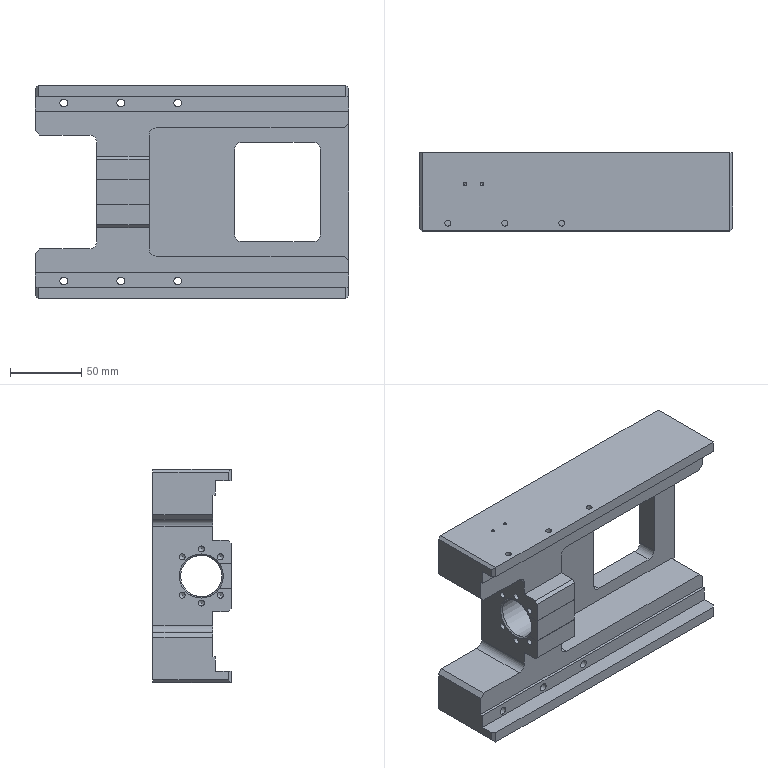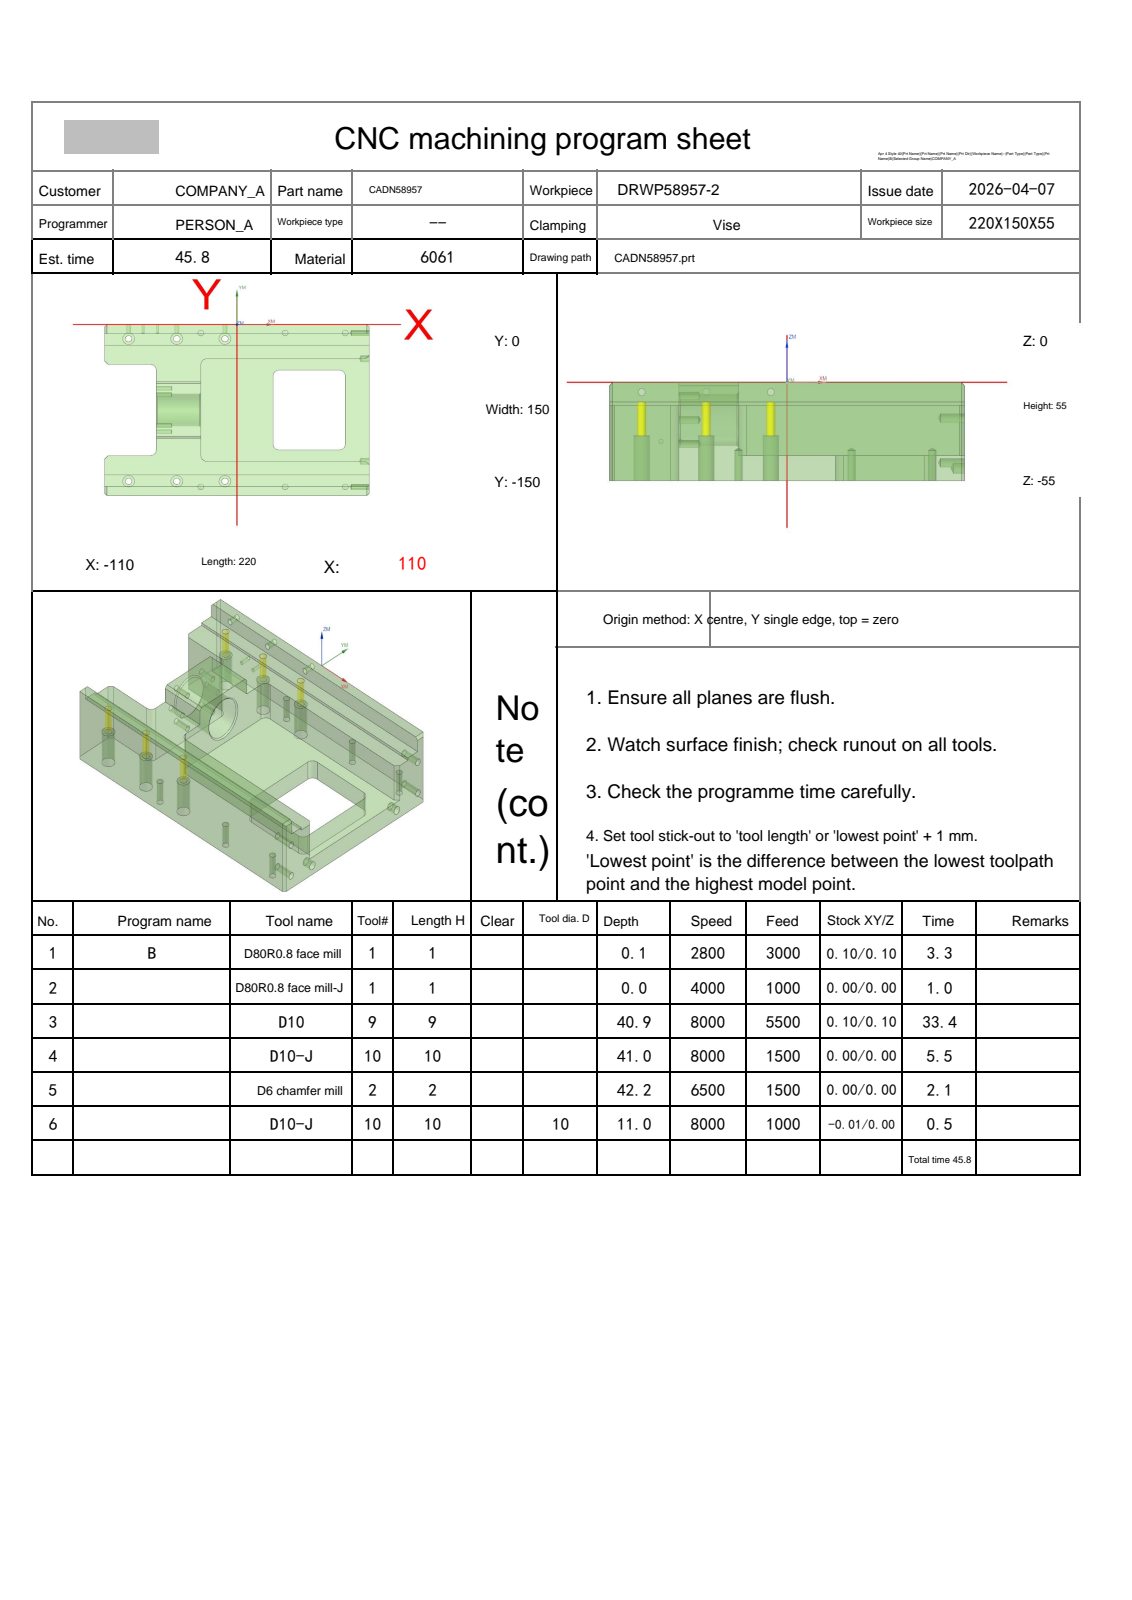NC program | NX | posted by the shop | part box 220 x 55 x 150 mm
Lines 209 to 1303 of 15484:
N3 T09 M06
(D10  D=10. R=0. H=09 ce=0.10 di=0.10)
G00 G90 G54 X124.5 Y-57.103 M03 S8000
G43 H09 Z14.5
M08
Z.519
G01 Z-.681 F5500.
X117.071 Y-57.1
X117.069
G03 X110.069 Y-64.097 I0.0 J-7.
G01 X110.05 Y-115.854
X110.06 Y-115.933
X109.985 Y-115.973
X109.925 Y-115.92
X109.712 Y-115.776
X108.83 Y-115.325
X108.229 Y-115.133
X107.955 Y-115.071
X107.072 Y-114.98
X-20.611 Y-114.978
G02 X-21.301 Y-114.701 I0.0 J1.
G01 X-24.423 Y-111.722
G03 X-25.113 Y-111.446 I-.69 J-.723
G01 X-25.209 Y-111.45
X-33.928 Y-112.288
G02 X-34.167 Y-112.299 I-.239 J2.489
X-36.667 Y-109.799 I0.0 J2.5
X-34.406 Y-107.311 I2.5 J0.0
G01 X-23.365 Y-106.25
G02 X-23.126 Y-106.239 I.239 J-2.489
X-20.626 Y-108.739 I0.0 J-2.5
X-21.254 Y-110.396 I-2.5 J0.0
G01 X-24.533 Y-114.678
G02 X-25.309 Y-115.07 I-.794 J.608
G01 X-25.877 Y-115.08
X-29.442
X-30.06 Y-115.142
X-29.576 Y-116.808
X-29.375 Y-117.251
X-29.126 Y-117.68
X-28.494 Y-118.464
X-28.401 Y-118.556
X-27.617 Y-119.166
X-27.132 Y-119.434
X-26.742 Y-119.601
X-25.862 Y-119.843
X-24.981 Y-119.92
X107.
X107.057 Y-119.943
X110.057 Y-122.943
X110.08 Y-123.
Y-126.698
X110.079 Y-127.517
X110.08 Y-135.647
Y-136.418
Y-136.823
G02 X114.225 Y-139.047 I-.107 J-5.175
X115.158 Y-142.351 I-5.386 J-3.304
X115.151 Y-142.651 I-6.318 J0.0
G01 Y-148.
X115.127 Y-148.057
X113.936 Y-149.248
X113.823
Y-142.
G03 X108.893 Y-136.904 I-5.121 J-.021
G01 X108.343 Y-136.832
X108.169 Y-136.822
X107.968 Y-136.821
X-104.399
X-105.291
X-107.968
X-108.173 Y-136.822
X-108.349 Y-136.832
X-108.894 Y-136.904
G03 X-113.823 Y-142. I.192 J-5.117
G01 Y-149.248
X-113.931 Y-149.249
X-115.127 Y-148.046
X-115.151 Y-147.99
Y-142.647
X-115.13 Y-141.755
G02 X-110.08 Y-136.824 I5.205 J-.279
G01 Y-136.418
Y-135.647
X-110.079 Y-127.517
X-110.08 Y-126.698
Y-118.
X-110.057 Y-117.943
X-107.057 Y-114.943
X-107. Y-114.92
X-72.278
X-70.917 Y-114.862
X-69.636 Y-114.315
X-69.279 Y-114.099
X-68.759 Y-113.701
X-68.513 Y-113.471
X-68.283 Y-113.224
X-67.881 Y-112.691
X-67.677 Y-112.349
X-67.136 Y-111.071
X-67.08 Y-109.713
Y-105.264
X-67.082 Y-105.086
X-67.081 Y-103.823
X-67.001
X-66.998
X-66.997
X-66.921 Y-103.824
X-37.336 Y-103.823
G02 X-36.336 Y-104.823 I0.0 J-1.
G01 X-36.35 Y-104.989
X-37.197 Y-110.005
X-37.211 Y-110.171
G03 X-36.775 Y-110.997 I1. J0.0
G02 X-36.339 Y-111.823 I-.564 J-.826
X-36.428 Y-112.235 I-1. J0.0
G03 X-37.06 Y-115.142 I6.368 J-2.907
X-36.782 Y-117.097 I7. J0.0
G01 X-36.157 Y-119.243
X-35.605 Y-120.461
X-34.911 Y-121.657
X-33.689 Y-123.173
X-33.019 Y-123.831
X-31.484 Y-125.027
X-30.211 Y-125.73
X-29.062 Y-126.223
X-27.105 Y-126.762
X-25.284 Y-126.92
X102.083
G02 X103.079 Y-127.916 I-.003 J-1.
G01 Y-128.825
G02 X102.083 Y-129.821 I-1. J.003
G01 X-64.065
G02 X-64.758 Y-129.542 I0.0 J1.
G01 X-66.167 Y-128.188
G03 X-66.65 Y-127.931 I-.693 J-.721
G02 X-68.627 Y-125.486 I.523 J2.445
X-66.82 Y-123.084 I2.5 J0.0
G01 X-59.894 Y-121.087
G02 X-59.202 Y-120.989 I.693 J-2.402
X-56.702 Y-123.489 I0.0 J-2.5
X-58.509 Y-125.891 I-2.5 J0.0
G01 X-64.219 Y-127.538
G03 X-64.7 Y-127.846 I.277 J-.961
G01 X-66.101 Y-129.474
G02 X-66.859 Y-129.821 I-.758 J.653
G01 X-102.083
G02 X-103.079 Y-128.825 I.003 J1.
G01 Y-127.514
X-103.08 Y-126.695
Y-122.916
G02 X-102.084 Y-121.92 I1. J-.004
G01 X-72.128
X-70.619 Y-121.856
G03 X-68.168 Y-121.299 I-.299 J6.994
G01 X-66.436 Y-120.559
X-65.332 Y-119.893
X-64.228 Y-119.049
X-63.548 Y-118.412
X-62.912 Y-117.726
X-62.065 Y-116.605
X-61.419 Y-115.522
X-60.69 Y-113.799
G03 X-60.167 Y-111.725 I-6.446 J2.729
G02 X-59.175 Y-110.823 I.995 J-.097
G01 X-40.813
G02 X-40.114 Y-111.523 I0.0 J-.7
X-40.151 Y-111.748 I-.7 J0.0
G01 X-43.004 Y-120.119
G03 X-43.057 Y-120.442 I.947 J-.322
X-43.018 Y-120.721 I1. J0.0
G01 X-42.778 Y-121.546
G02 X-42.739 Y-121.821 I-.961 J-.275
X-43.735 Y-122.821 I-1. J0.0
G01 X-55.984
G02 X-56.98 Y-121.821 I.004 J1.
X-56.78 Y-121.222 I1. J0.0
G01 X-56.249 Y-120.518
X-55.161 Y-118.695
X-55.048 Y-118.429
G02 X-54.133 Y-117.823 I.919 J-.394
G01 X-46.706
G03 X-46.094 Y-117.613 I0.0 J1.
G01 X-37.808 Y-111.189
G03 X-37.421 Y-110.399 I-.613 J.79
G01 X-37.435 Y-110.233
X-38.322 Y-104.989
X-38.336 Y-104.823
G02 X-37.336 Y-103.823 I1. J0.0
G01 X-30.
G03 X-24.905 Y-98.909 I-.049 J5.149
G01 X-24.865 Y-98.686
X-24.822 Y-98.143
X-24.821 Y-97.253
Y-52.747
X-24.822 Y-51.851
X-24.866 Y-51.305
X-24.905 Y-51.091
G03 X-30. Y-46.177 I-5.144 J-.235
G01 X-66.921
X-66.997
X-66.998
X-67.001
X-67.002
X-67.081
X-67.082 Y-44.898
X-67.08 Y-40.287
X-67.136 Y-38.929
X-67.677 Y-37.651
X-67.881 Y-37.309
X-68.283 Y-36.777
X-68.76 Y-36.298
X-69.279 Y-35.901
X-69.636 Y-35.685
X-70.917 Y-35.138
X-72.278 Y-35.08
X-107.
X-107.057 Y-35.057
X-110.057 Y-32.057
X-110.08 Y-32.
Y-23.302
X-110.079 Y-22.483
X-110.08 Y-14.353
Y-13.176
G02 X-112.672 Y-12.396 I.155 J5.21
X-115.13 Y-8.242 I2.748 J4.43
G01 X-115.151 Y-6.461
Y-2.
X-115.127 Y-1.943
X-113.935 Y-.751
X-113.823 Y-.752
X-113.822 Y-8.068
G03 X-108.895 Y-13.096 I5.12 J.088
G01 X-108.343 Y-13.168
X-108.169 Y-13.178
X-7.311 Y-13.179
X99.045
X99.937 Y-13.18
X101.722
X102.168
X102.614
X103.507
X104.399
X105.291
X108.004 Y-13.177
X108.173 Y-13.178
X108.349 Y-13.168
X108.894 Y-13.096
G03 X113.823 Y-8. I-.192 J5.117
G01 Y-.752
X113.932
X115.127 Y-1.954
X115.151 Y-2.01
Y-6.462
X115.13 Y-8.245
G02 X113. Y-12.174 I-5.206 J.28
X110.08 Y-13.177 I-3.077 J4.209
G01 X110.079 Y-22.483
X110.08 Y-23.302
Y-26.967
X113. Y-29.888
Y-31.328
X110.698 Y-33.63
X110.143 Y-34.118
X110.08 Y-34.166
X110.07 Y-61.083
G02 X109.651 Y-61.896 I-1. J.001
G01 X103.486 Y-66.296
G03 X103.068 Y-67.109 I.581 J-.814
G01 X103.053 Y-106.984
G02 X102.057 Y-107.98 I-1. J.004
G01 X-19.858 Y-107.978
G02 X-20.854 Y-106.978 I.003 J1.
X-20.632 Y-106.349 I1. J0.0
G03 X-17.951 Y-99.781 I-9.418 J7.676
X-17.887 Y-99.24 I-6.994 J1.101
G01 X-17.844 Y-98.703
G03 X-17.822 Y-98.143 I-7.058 J.56
G01 Y-51.857
G03 X-17.844 Y-51.297 I-7.08 J0.0
G01 X-17.887 Y-50.76
G03 X-17.951 Y-50.219 I-7.058 J-.56
X-29.966 Y-39.177 I-12.099 J-1.108
G01 X-59.175
G02 X-60.167 Y-38.275 I.003 J1.
G03 X-60.69 Y-36.201 I-6.969 J-.655
G01 X-61.419 Y-34.478
X-62.065 Y-33.395
X-62.368 Y-32.995
X-62.985 Y-32.177
X-64.133 Y-31.024
X-65.332 Y-30.107
X-66.436 Y-29.441
X-68.168 Y-28.701
G03 X-70.619 Y-28.144 I-2.749 J-6.437
G01 X-72.128 Y-28.08
X-102.084
G02 X-103.08 Y-27.083 I.004 J1.
G01 Y-23.305
X-103.079 Y-22.486
Y-21.174
G02 X-102.083 Y-20.178 I1. J-.003
G01 X-66.86
G02 X-66.102 Y-20.526 I0.0 J-1.
G01 X-64.7 Y-22.153
G03 X-64.22 Y-22.462 I.758 J.653
G01 X-58.509 Y-24.108
G02 X-56.702 Y-26.511 I-.693 J-2.402
X-59.202 Y-29.011 I-2.5 J0.0
X-59.894 Y-28.913 I0.0 J2.5
G01 X-66.82 Y-26.915
G02 X-68.627 Y-24.513 I.693 J2.402
X-66.651 Y-22.069 I2.5 J0.0
G03 X-66.167 Y-21.812 I-.209 J.978
G01 X-64.758 Y-20.457
G02 X-64.065 Y-20.178 I.693 J-.721
G01 X-7.311 Y-20.179
X99.041
X99.933 Y-20.18
X101.721
X102.083
G02 X103.079 Y-21.177 I-.004 J-1.
G01 Y-22.486
X103.08 Y-23.305
Y-26.967
G03 X103.83 Y-30.12 I7. J0.0
G02 X103.935 Y-30.567 I-.895 J-.447
X103.83 Y-31.014 I-1. J0.0
G03 X103.08 Y-34.163 I6.25 J-3.152
G01 X103.07 Y-61.081
G02 X102.651 Y-61.894 I-1. J.001
G01 X96.486 Y-66.294
G03 X96.068 Y-67.106 I.581 J-.814
G01 X96.056 Y-99.984
G02 X95.06 Y-100.98 I-1. J.004
G01 X-9.924 Y-100.978
G02 X-10.92 Y-99.978 I.004 J1.
G01 X-10.917 Y-99.896
X-10.866 Y-99.257
G03 X-10.822 Y-98.143 I-14.036 J1.114
G01 Y-51.857
G03 X-10.866 Y-50.743 I-14.08 J0.0
G01 X-10.909 Y-50.206
G03 X-11. Y-49.368 I-14.036 J-1.114
X-29.942 Y-32.177 I-19.049 J-1.959
G01 X-54.133
G02 X-55.048 Y-31.571 I.004 J1.
G01 X-55.161 Y-31.305
X-56.249 Y-29.482
X-56.78 Y-28.778
G02 X-56.98 Y-28.178 I.801 J.599
X-55.984 Y-27.178 I1. J0.0
G01 X-18.168 Y-27.179
G02 X-17.401 Y-27.538 I0.0 J-1.
G01 X-16.08 Y-29.12
G03 X-15.642 Y-29.424 I.768 J.641
G01 X-10.619 Y-31.176
G02 X-8.942 Y-33.536 I-.823 J-2.361
X-11.442 Y-36.036 I-2.5 J0.0
X-12.266 Y-35.897 I0.0 J2.5
G01 X-18.423 Y-33.749
G02 X-20.099 Y-31.389 I.823 J2.361
X-17.97 Y-28.916 I2.5 J0.0
G03 X-17.437 Y-28.658 I-.148 J.989
G01 X-16.139 Y-27.448
G02 X-15.457 Y-27.179 I.682 J-.731
G01 X-7.311
X95.133
G02 X96.125 Y-28.094 I-.004 J-1.
G03 X96.49 Y-30.331 I13.955 J1.127
G02 X96.518 Y-30.567 I-.972 J-.236
X96.49 Y-30.803 I-1. J0.0
G03 X96.08 Y-34.166 I13.59 J-3.363
G01 Y-34.179
X96.07 Y-61.078
G02 X95.651 Y-61.891 I-1. J.001
G01 X89.486 Y-66.291
G03 X89.068 Y-67.104 I.581 J-.814
G01 X89.058 Y-92.984
G02 X88.063 Y-93.98 I-1. J.005
G01 X-2.826 Y-93.978
G02 X-3.822 Y-92.983 I.004 J1.
G01 Y-51.857
G03 X-3.888 Y-50.19 I-21.08 J0.0
G01 X-3.931 Y-49.652
G03 X-4.05 Y-48.527 I-21.014 J-1.668
X-9.03 Y-35.77 I-25.999 J-2.799
G02 X-9.224 Y-35.179 I.807 J.591
X-8.228 Y-34.179 I1. J0.0
G01 X-7.311
X88.084
G02 X89.08 Y-35.175 I-.004 J-1.
G01 X89.07 Y-61.076
G02 X88.651 Y-61.888 I-1. J.001
G01 X82.487 Y-66.288
G03 X82.068 Y-67.101 I.581 J-.814
G01 X82.061 Y-85.985
G02 X81.066 Y-86.979 I-1. J.005
G01 X4.173 Y-86.978
G02 X3.178 Y-85.983 I.005 J1.
G01 Y-51.856
G03 X3.09 Y-49.636 I-28.08 J0.0
G01 X3.048 Y-49.098
G03 X2.9 Y-47.69 I-27.992 J-2.222
X1.887 Y-42.442 I-32.949 J-3.637
G02 X1.852 Y-42.179 I.965 J.263
X2.847 Y-41.179 I1. J0.0
G01 X81.082
G02 X82.077 Y-42.174 I-.005 J-1.
G01 X82.07 Y-61.073
G02 X81.651 Y-61.886 I-1. J.001
G01 X75.487 Y-66.286
G03 X75.068 Y-67.099 I.581 J-.814
G01 X75.063 Y-78.985
G02 X74.068 Y-79.979 I-1. J.005
G01 X11.173 Y-79.978
G02 X10.178 Y-78.983 I.005 J1.
G01 Y-51.856
G03 X10.081 Y-49.248 I-35.08 J-.001
G01 X10.079 Y-49.179
G02 X11.074 Y-48.179 I1. J0.0
G01 X74.079
G02 X75.074 Y-49.174 I-.005 J-1.
G01 X75.07 Y-61.07
G02 X74.651 Y-61.883 I-1. J.001
G01 X68.487 Y-66.283
G03 X68.068 Y-67.096 I.581 J-.814
G01 X68.066 Y-71.985
G02 X67.071 Y-72.979 I-1. J.005
G01 X18.173
G02 X17.178 Y-71.984 I.005 J1.
G01 Y-56.174
G02 X18.173 Y-55.179 I1. J-.005
G01 X67.077
G02 X68.072 Y-56.174 I-.005 J-1.
G01 X68.07 Y-60.957
G02 X67.507 Y-61.855 I-1. J.001
G01 X61.508 Y-64.771
G03 X61.007 Y-65.325 I.438 J-.899
G02 X60.074 Y-65.979 I-.938 J.345
G01 X25.173
G02 X24.178 Y-64.984 I.005 J1.
G01 Y-63.174
G02 X25.173 Y-62.179 I1. J-.005
G01 X60.074
G02 X61.069 Y-63.174 I-.005 J-1.
G01 Y-64.079
Y-64.579
Y-64.582
G03 X68.066 Y-71.582 I7. J0.0
G01 Z.519
G00 Z3.
G01 X124.5 Y-57.103 F6000.
G00 Z-.163
G01 Z-1.363 F5500.
X117.071 Y-57.1
X117.069
G03 X110.069 Y-64.097 I0.0 J-7.
G01 X110.05 Y-115.854
X110.06 Y-115.933
X109.985 Y-115.973
X109.925 Y-115.92
X109.712 Y-115.776
X108.83 Y-115.325
X108.229 Y-115.133
X107.955 Y-115.071
X107.072 Y-114.98
X-20.031 Y-114.978
G02 X-20.718 Y-114.705 I0.0 J1.
G01 X-23.701 Y-111.886
G03 X-24.387 Y-111.612 I-.687 J-.727
G01 X-24.504 Y-111.619
X-34.254 Y-112.76
G02 X-34.545 Y-112.777 I-.291 J2.483
X-37.045 Y-110.277 I0.0 J2.5
X-34.835 Y-107.794 I2.5 J0.0
G01 X-22.821 Y-106.388
G02 X-22.531 Y-106.371 I.291 J-2.483
X-20.031 Y-108.871 I0.0 J-2.5
X-20.667 Y-110.538 I-2.5 J0.0
G01 X-23.752 Y-114.584
G02 X-24.547 Y-114.978 I-.795 J.606
G01 X-24.819
X-24.943 Y-115.053
X-24.983 Y-115.064
X-25.877 Y-115.08
X-29.442
X-30.06 Y-115.142
X-29.576 Y-116.808
X-29.375 Y-117.251
X-29.126 Y-117.68
X-28.494 Y-118.464
X-28.401 Y-118.556
X-27.617 Y-119.166
X-27.132 Y-119.434
X-26.742 Y-119.601
X-25.862 Y-119.843
X-24.981 Y-119.92
X107.
X107.057 Y-119.943
X110.057 Y-122.943
X110.08 Y-123.
Y-126.698
X110.079 Y-127.517
X110.08 Y-136.418
Y-136.823
G02 X114.225 Y-139.047 I-.107 J-5.175
X115.158 Y-142.351 I-5.386 J-3.304
X115.151 Y-142.651 I-6.318 J0.0
G01 Y-148.
X115.127 Y-148.057
X114.617 Y-148.567
X114.504
Y-142.
G03 X109.383 Y-136.9 I-5.121 J-.021
G01 X109.362
X108.878
X108.343 Y-136.832
X108.169 Y-136.822
X107.968 Y-136.821
X-104.399
X-105.292
X-107.968
X-108.173 Y-136.822
X-108.349 Y-136.832
X-108.878 Y-136.9
X-109.367
G03 X-114.504 Y-142.037 I0.0 J-5.137
G01 Y-148.567
X-114.609
X-115.127 Y-148.046
X-115.151 Y-147.99
Y-142.647
X-115.13 Y-141.755
G02 X-110.08 Y-136.824 I5.205 J-.279
G01 Y-136.418
X-110.079 Y-127.517
X-110.08 Y-126.698
Y-118.
X-110.057 Y-117.943
X-107.057 Y-114.943
X-107. Y-114.92
X-72.278
X-70.917 Y-114.862
X-69.636 Y-114.315
X-69.279 Y-114.099
X-68.759 Y-113.701
X-68.513 Y-113.471
X-68.283 Y-113.224
X-67.881 Y-112.691
X-67.677 Y-112.349
X-67.136 Y-111.071
X-67.08 Y-109.713
Y-105.264
X-67.082 Y-105.086
X-67.081 Y-104.504
X-67.051
X-67.05 Y-104.505
X-67.001 Y-104.504
X-66.921 Y-104.505
X-37.609 Y-104.504
G02 X-36.609 Y-105.504 I0.0 J-1.
G01 X-36.623 Y-105.671
X-37.471 Y-110.686
X-37.485 Y-110.852
G03 X-37.049 Y-111.678 I1. J0.0
G02 X-36.613 Y-112.504 I-.564 J-.826
X-36.668 Y-112.831 I-1. J0.0
G03 X-37.06 Y-115.142 I6.607 J-2.311
X-36.782 Y-117.097 I7. J0.0
G01 X-36.157 Y-119.243
X-35.605 Y-120.461
X-34.911 Y-121.657
X-33.689 Y-123.173
X-33.019 Y-123.831
X-31.484 Y-125.027
X-30.211 Y-125.73
X-29.062 Y-126.223
X-27.105 Y-126.762
X-25.284 Y-126.92
X102.083
G02 X103.079 Y-127.916 I-.003 J-1.
G01 Y-128.825
G02 X102.083 Y-129.821 I-1. J.003
G01 X-64.065
G02 X-64.758 Y-129.542 I0.0 J1.
G01 X-66.167 Y-128.188
G03 X-66.65 Y-127.931 I-.693 J-.721
G02 X-68.627 Y-125.486 I.523 J2.445
X-66.82 Y-123.084 I2.5 J0.0
G01 X-59.894 Y-121.087
G02 X-59.202 Y-120.989 I.693 J-2.402
X-56.702 Y-123.489 I0.0 J-2.5
X-58.509 Y-125.891 I-2.5 J0.0
G01 X-64.219 Y-127.538
G03 X-64.7 Y-127.846 I.277 J-.961
G01 X-66.101 Y-129.474
G02 X-66.859 Y-129.821 I-.758 J.653
G01 X-102.083
G02 X-103.079 Y-128.825 I.003 J1.
G01 Y-127.514
X-103.08 Y-126.695
Y-122.916
G02 X-102.084 Y-121.92 I1. J-.004
G01 X-72.128
X-70.619 Y-121.856
G03 X-68.168 Y-121.299 I-.299 J6.994
G01 X-66.436 Y-120.559
X-65.332 Y-119.893
X-64.228 Y-119.049
X-63.548 Y-118.412
X-62.912 Y-117.726
X-62.065 Y-116.605
X-61.419 Y-115.522
X-60.69 Y-113.799
G03 X-60.249 Y-112.322 I-6.446 J2.729
G02 X-59.269 Y-111.504 I.983 J-.182
G01 X-41.044
G02 X-40.344 Y-112.204 I0.0 J-.7
G01 X-40.373 Y-112.401
X-42.835 Y-120.785
G03 X-42.876 Y-121.067 I.96 J-.281
X-42.836 Y-121.346 I1. J0.0
G01 X-42.778 Y-121.546
G02 X-42.739 Y-121.821 I-.961 J-.275
X-43.735 Y-122.821 I-1. J0.0
G01 X-55.984
G02 X-56.98 Y-121.821 I.004 J1.
X-56.78 Y-121.222 I1. J0.0
G01 X-56.249 Y-120.518
X-55.336 Y-118.988
G02 X-54.483 Y-118.504 I.857 J-.516
G01 X-46.564
G03 X-45.933 Y-118.28 I0.0 J1.
G01 X-38.061 Y-111.871
G03 X-37.692 Y-111.096 I-.632 J.775
G01 X-37.706 Y-110.93
X-38.595 Y-105.671
X-38.609 Y-105.504
G02 X-37.609 Y-104.504 I1. J0.0
G01 X-30.
G03 X-24.9 Y-99.383 I-.021 J5.121
G01 Y-99.362
Y-98.88
X-24.865 Y-98.686
X-24.822 Y-98.143
X-24.821 Y-97.253
Y-52.747
X-24.822 Y-51.851
X-24.866 Y-51.305
X-24.9 Y-51.12
Y-50.615
G03 X-30. Y-45.496 I-5.121 J-.002
G01 X-66.921
X-67.001
Y-45.495
X-67.081 Y-45.496
X-67.082 Y-44.898
X-67.08 Y-40.287
X-67.136 Y-38.929
X-67.677 Y-37.651
X-67.881 Y-37.309
X-68.283 Y-36.777
X-68.76 Y-36.298
X-69.279 Y-35.901
X-69.636 Y-35.685
X-70.917 Y-35.138
X-72.278 Y-35.08
X-107.
X-107.057 Y-35.057
X-110.057 Y-32.057
X-110.08 Y-32.
Y-23.302
X-110.079 Y-22.483
X-110.08 Y-14.461
Y-13.176
G02 X-115.13 Y-8.242 I.155 J5.21
G01 X-115.151 Y-6.461
Y-2.
X-115.127 Y-1.943
X-114.617 Y-1.433
X-114.504
Y-7.963
G03 X-109.367 Y-13.1 I5.137 J0.0
G01 X-108.879
X-108.343 Y-13.168
X-108.169 Y-13.178
X-7.311 Y-13.179
X99.045
X99.937 Y-13.18
X101.722
X102.614
X103.507
X104.399
X105.291
X108.004 Y-13.177
X108.173 Y-13.178
X108.349 Y-13.168
X108.879 Y-13.1
X109.362
X109.383
G03 X114.504 Y-8. I0.0 J5.121
G01 Y-1.433
X114.609
X115.127 Y-1.954
X115.151 Y-2.01
Y-6.462
X115.13 Y-8.245
G02 X110.08 Y-13.176 I-5.206 J.28
G01 X110.079 Y-22.483
X110.08 Y-23.302
Y-26.967
X113. Y-29.888
Y-31.328
X110.698 Y-33.63
X110.143 Y-34.118
X110.08 Y-34.166
X110.07 Y-61.083
G02 X109.651 Y-61.896 I-1. J.001
G01 X103.486 Y-66.296
G03 X103.068 Y-67.109 I.581 J-.814
G01 X103.053 Y-106.984
G02 X102.057 Y-107.98 I-1. J.004
G01 X-19.325 Y-107.978
G02 X-20.322 Y-106.978 I.004 J1.
X-20.139 Y-106.402 I1. J0.0
G03 X-17.9 Y-99.388 I-9.882 J7.019
G01 X-17.881 Y-99.17
X-17.844 Y-98.703
G03 X-17.822 Y-98.143 I-7.058 J.56
G01 Y-51.857
G03 X-17.844 Y-51.297 I-7.08 J0.0
G01 X-17.887 Y-50.76
X-17.9 Y-50.612
G03 X-29.986 Y-38.496 I-12.121 J-.005
G01 X-59.269
G02 X-60.249 Y-37.678 I.003 J1.
G03 X-60.69 Y-36.201 I-6.887 J-1.251
G01 X-61.419 Y-34.478
X-62.065 Y-33.395
X-62.984 Y-32.178
X-64.133 Y-31.024
X-65.332 Y-30.107
X-66.436 Y-29.441
X-68.168 Y-28.701
G03 X-70.619 Y-28.144 I-2.749 J-6.437
G01 X-72.128 Y-28.08
X-102.084
G02 X-103.08 Y-27.084 I.003 J1.
G01 Y-23.305
X-103.079 Y-22.486
Y-21.174
G02 X-102.083 Y-20.178 I1. J-.003
G01 X-66.86
G02 X-66.102 Y-20.526 I0.0 J-1.
G01 X-64.7 Y-22.153
G03 X-64.22 Y-22.462 I.758 J.653
G01 X-58.509 Y-24.108
G02 X-56.702 Y-26.511 I-.693 J-2.402
X-59.202 Y-29.011 I-2.5 J0.0
X-59.894 Y-28.913 I0.0 J2.5
G01 X-66.82 Y-26.915
G02 X-68.627 Y-24.513 I.693 J2.402
X-66.651 Y-22.069 I2.5 J0.0
G03 X-66.167 Y-21.812 I-.209 J.978
G01 X-64.758 Y-20.457
G02 X-64.065 Y-20.178 I.693 J-.721
G01 X-7.311 Y-20.179
X99.041
X99.933 Y-20.18
X101.721
X102.083
G02 X103.079 Y-21.177 I-.004 J-1.
G01 Y-22.486
X103.08 Y-23.305
Y-26.967
G03 X103.83 Y-30.12 I7. J0.0
G02 X103.935 Y-30.567 I-.895 J-.447
X103.83 Y-31.014 I-1. J0.0
G03 X103.08 Y-34.163 I6.25 J-3.152
G01 X103.07 Y-61.081
G02 X102.651 Y-61.894 I-1. J.001
G01 X96.486 Y-66.294
G03 X96.068 Y-67.106 I.581 J-.814
G01 X96.056 Y-99.984
G02 X95.06 Y-100.98 I-1. J.004
G01 X-9.913 Y-100.978
G02 X-10.909 Y-99.978 I.004 J1.
G01 X-10.908 Y-99.953
X-10.903 Y-99.724
X-10.866 Y-99.257
G03 X-10.822 Y-98.144 I-14.036 J1.114
G01 Y-51.856
G03 X-10.866 Y-50.743 I-14.08 J0.0
G01 X-10.903 Y-50.276
G03 X-29.976 Y-31.496 I-19.118 J-.341
G01 X-54.483
G02 X-55.336 Y-31.012 I.004 J1.
G01 X-56.249 Y-29.482
X-56.78 Y-28.778
G02 X-56.98 Y-28.178 I.801 J.599
X-55.984 Y-27.178 I1. J0.0
G01 X-17.235 Y-27.179
G02 X-16.464 Y-27.542 I0.0 J-1.
G01 X-15.169 Y-29.11
G03 X-14.745 Y-29.411 I.771 J.637
G01 X-10.05 Y-31.148
G02 X-8.417 Y-33.493 I-.867 J-2.345
X-10.917 Y-35.993 I-2.5 J0.0
X-11.785 Y-35.838 I0.0 J2.5
G01 X-17.587 Y-33.691
G02 X-19.22 Y-31.346 I.867 J2.345
X-17.04 Y-28.867 I2.5 J0.0
G03 X-16.489 Y-28.609 I-.128 J.992
G01 X-15.229 Y-27.445
G02 X-14.55 Y-27.179 I.679 J-.734
G01 X-7.311
X95.133
G02 X96.125 Y-28.094 I-.004 J-1.
G03 X96.49 Y-30.331 I13.955 J1.127
G02 X96.518 Y-30.567 I-.972 J-.236
X96.49 Y-30.803 I-1. J0.0
G03 X96.08 Y-34.166 I13.59 J-3.363
G01 Y-34.179
X96.07 Y-61.078
G02 X95.651 Y-61.891 I-1. J.001
G01 X89.486 Y-66.291
G03 X89.068 Y-67.104 I.581 J-.814
G01 X89.058 Y-92.984
G02 X88.063 Y-93.98 I-1. J.005
G01 X-2.826 Y-93.978
G02 X-3.822 Y-92.983 I.004 J1.
G01 Y-51.856
G03 X-3.888 Y-50.189 I-21.08 J-.001
G01 X-3.909 Y-49.92
G03 X-8.547 Y-35.745 I-26.111 J-.697
G02 X-8.722 Y-35.179 I.825 J.566
X-7.727 Y-34.179 I1. J0.0
G01 X-7.311
X88.084
G02 X89.08 Y-35.175 I-.004 J-1.
G01 X89.07 Y-61.076
G02 X88.651 Y-61.888 I-1. J.001
G01 X82.487 Y-66.288
G03 X82.068 Y-67.101 I.581 J-.814
G01 X82.061 Y-85.985
G02 X81.066 Y-86.979 I-1. J.005
G01 X4.173 Y-86.978
G02 X3.178 Y-85.983 I.005 J1.
G01 Y-51.856
Y-51.855
G03 X3.082 Y-49.539 I-28.08 J0.0
X2.07 Y-42.422 I-33.103 J-1.078
G02 X2.04 Y-42.179 I.97 J.243
X3.036 Y-41.179 I1. J0.0
G01 X81.082
G02 X82.077 Y-42.174 I-.005 J-1.
G01 X82.07 Y-61.073
G02 X81.651 Y-61.886 I-1. J.001
G01 X75.487 Y-66.286
G03 X75.068 Y-67.099 I.581 J-.814
G01 X75.063 Y-78.985
G02 X74.068 Y-79.979 I-1. J.005
G01 X11.173 Y-79.978
G02 X10.178 Y-78.983 I.005 J1.
G01 Y-51.856
Y-51.855
G03 X10.081 Y-49.248 I-35.08 J0.0
G01 X10.079 Y-49.179
G02 X11.074 Y-48.179 I1. J0.0
G01 X74.079
G02 X75.074 Y-49.174 I-.005 J-1.
G01 X75.07 Y-61.07
G02 X74.651 Y-61.883 I-1. J.001
G01 X68.487 Y-66.283
G03 X68.068 Y-67.096 I.581 J-.814
G01 X68.066 Y-71.985
G02 X67.071 Y-72.979 I-1. J.005
G01 X18.173
G02 X17.178 Y-71.984 I.005 J1.
G01 Y-56.174
G02 X18.173 Y-55.179 I1. J-.005
G01 X67.077
G02 X68.072 Y-56.174 I-.005 J-1.
G01 X68.07 Y-60.957
G02 X67.507 Y-61.855 I-1. J.001
G01 X61.508 Y-64.771
G03 X61.007 Y-65.325 I.438 J-.899
G02 X60.074 Y-65.979 I-.938 J.345
G01 X25.173
G02 X24.178 Y-64.984 I.005 J1.
G01 Y-63.174
G02 X25.173 Y-62.179 I1. J-.005
G01 X60.074
G02 X61.069 Y-63.174 I-.005 J-1.
G01 Y-64.079
Y-64.579
Y-64.582
G03 X68.066 Y-71.582 I7. J0.0
G01 Z-.163
G00 Z3.
G01 X124.5 Y-57.103 F6000.
G00 Z-.844
G01 Z-2.044 F5500.
X117.071 Y-57.1
X117.069
G03 X110.069 Y-64.097 I0.0 J-7.
G01 X110.05 Y-115.854
X110.06 Y-115.933
X109.985 Y-115.973
X109.925 Y-115.92
X109.712 Y-115.776
X108.83 Y-115.325
X108.229 Y-115.133
X107.955 Y-115.071
X107.072 Y-114.98
X-24.819 Y-114.978
X-24.943 Y-115.053
X-24.983 Y-115.064
X-25.877 Y-115.08
X-28.506
G02 X-29.018 Y-114.939 I0.0 J1.
G01 X-32.536 Y-112.84
X-32.673 Y-112.772
G02 X-34.235 Y-110.454 I.937 J2.318
X-32.125 Y-107.985 I2.5 J0.0
G01 X-22.463 Y-106.46
G02 X-22.074 Y-106.43 I.39 J-2.469
X-19.574 Y-108.93 I0.0 J-2.5
X-21.684 Y-111.399 I-2.5 J0.0
G01 X-29.228 Y-112.589
G03 X-30.073 Y-113.577 I.156 J-.988
G01 Y-113.585
X-30.061 Y-115.004
G03 X-30.022 Y-115.275 I1. J.008
G01 X-29.576 Y-116.808
X-29.375 Y-117.251
X-29.126 Y-117.68
X-28.494 Y-118.464
X-28.401 Y-118.556
X-27.617 Y-119.166
X-27.132 Y-119.434
X-26.742 Y-119.601
X-25.862 Y-119.843
X-24.981 Y-119.92
X107.
X107.057 Y-119.943
X110.057 Y-122.943
X110.08 Y-123.
Y-126.698
X110.079 Y-127.517
X110.08 Y-136.418
Y-136.823
X109.92 Y-136.899
X109.404 Y-136.9
X109.401
X109.365
X109.362
X108.878
X108.747 Y-136.883
X108.343 Y-136.832
X108.169 Y-136.822
X107.968 Y-136.821
X-104.399
X-104.845
X-105.291
X-107.968
X-108.173 Y-136.822
X-108.349 Y-136.832
X-108.561 Y-136.859
X-108.878 Y-136.9
X-109.92
X-110.08 Y-136.824
Y-136.418
X-110.079 Y-127.517
X-110.08 Y-126.698
Y-118.
X-110.057 Y-117.943
X-107.057 Y-114.943
X-107. Y-114.92
X-72.278
X-70.917 Y-114.862
X-69.636 Y-114.315
X-69.279 Y-114.099
X-68.759 Y-113.701
X-68.513 Y-113.471
X-68.283 Y-113.224
X-67.881 Y-112.691
X-67.677 Y-112.349
X-67.136 Y-111.071
X-67.08 Y-109.713
Y-105.264
Y-105.105
X-66.92 Y-105.101
X-37.791 Y-105.1
G02 X-36.791 Y-106.1 I0.0 J-1.
G01 X-36.805 Y-106.267
X-37.653 Y-111.282
X-37.667 Y-111.449
G03 X-37.231 Y-112.274 I1. J0.0
G02 X-36.795 Y-113.1 I-.564 J-.826
X-36.828 Y-113.352 I-1. J0.0
G03 X-37.06 Y-115.142 I6.767 J-1.79
X-36.782 Y-117.097 I7. J0.0
G01 X-36.157 Y-119.243
X-35.605 Y-120.461
X-34.911 Y-121.657
X-33.689 Y-123.173
X-33.019 Y-123.831
X-31.484 Y-125.027
X-30.211 Y-125.73
X-29.062 Y-126.223
X-27.105 Y-126.762
X-25.284 Y-126.92
X102.083
G02 X103.079 Y-127.916 I-.004 J-1.
G01 Y-128.825
G02 X102.083 Y-129.821 I-1. J.004
G01 X-64.065
G02 X-64.758 Y-129.542 I0.0 J1.
G01 X-66.167 Y-128.188
G03 X-66.65 Y-127.931 I-.693 J-.721
G02 X-68.627 Y-125.486 I.523 J2.445
X-66.82 Y-123.084 I2.5 J0.0
G01 X-59.894 Y-121.087
G02 X-59.202 Y-120.989 I.693 J-2.402
X-56.702 Y-123.489 I0.0 J-2.5
X-58.509 Y-125.891 I-2.5 J0.0
G01 X-64.219 Y-127.538
G03 X-64.7 Y-127.846 I.277 J-.961
G01 X-66.101 Y-129.474
G02 X-66.859 Y-129.821 I-.758 J.653
G01 X-102.083
G02 X-103.079 Y-128.825 I.004 J1.
G01 Y-127.514
X-103.08 Y-126.695
Y-122.916
G02 X-102.084 Y-121.92 I1. J-.004
G01 X-72.128
X-70.619 Y-121.856
G03 X-68.168 Y-121.299 I-.299 J6.994
G01 X-66.436 Y-120.559
X-65.332 Y-119.893
X-64.228 Y-119.049
X-63.548 Y-118.412
X-62.912 Y-117.726
X-62.065 Y-116.605
X-61.419 Y-115.522
X-60.69 Y-113.799
G03 X-60.364 Y-112.843 I-6.446 J2.729
G02 X-59.401 Y-112.1 I.966 J-.257
G01 X-41.195
G02 X-40.495 Y-112.8 I0.0 J-.7
G01 X-40.518 Y-112.975
X-42.71 Y-121.46
G03 X-42.742 Y-121.71 I.968 J-.25
G01 X-42.741 Y-121.766
X-42.739 Y-121.821
G02 X-43.735 Y-122.821 I-1. J0.0
G01 X-55.984
G02 X-56.98 Y-121.821 I.004 J1.
X-56.78 Y-121.222 I1. J0.0
G01 X-56.249 Y-120.518
X-55.691 Y-119.584
G02 X-54.839 Y-119.1 I.857 J-.516
G01 X-46.427
G03 X-45.782 Y-118.863 I0.0 J1.
G01 X-38.226 Y-112.468
G03 X-37.872 Y-111.705 I-.646 J.763
G01 X-37.886 Y-111.539
X-38.778 Y-106.267
X-38.791 Y-106.1
G02 X-37.791 Y-105.1 I1. J0.0
G01 X-30.
G03 X-28.52 Y-104.88 I0.0 J5.1
G02 X-28.23 Y-104.837 I.29 J-.957
X-27.296 Y-105.48 I0.0 J-1.
G01 X-26.645 Y-107.181
G03 X-26.221 Y-107.684 I.934 J.357
G02 X-24.995 Y-109.835 I-1.274 J-2.151
X-27.22 Y-112.32 I-2.5 J0.0
G01 X-34.555 Y-113.133
G02 X-34.831 Y-113.148 I-.275 J2.485
X-37.331 Y-110.648 I0.0 J2.5
X-35.106 Y-108.163 I2.5 J0.0
G01 X-30.046 Y-107.602
G03 X-29.157 Y-106.608 I-.11 J.994
G01 X-29.163 Y-106.499
X-29.224 Y-105.947
X-29.23 Y-105.837
G02 X-28.52 Y-104.88 I1. J0.0
G03 X-24.9 Y-100. I-1.48 J4.88
G01 Y-98.88
X-24.865 Y-98.686
X-24.822 Y-98.143